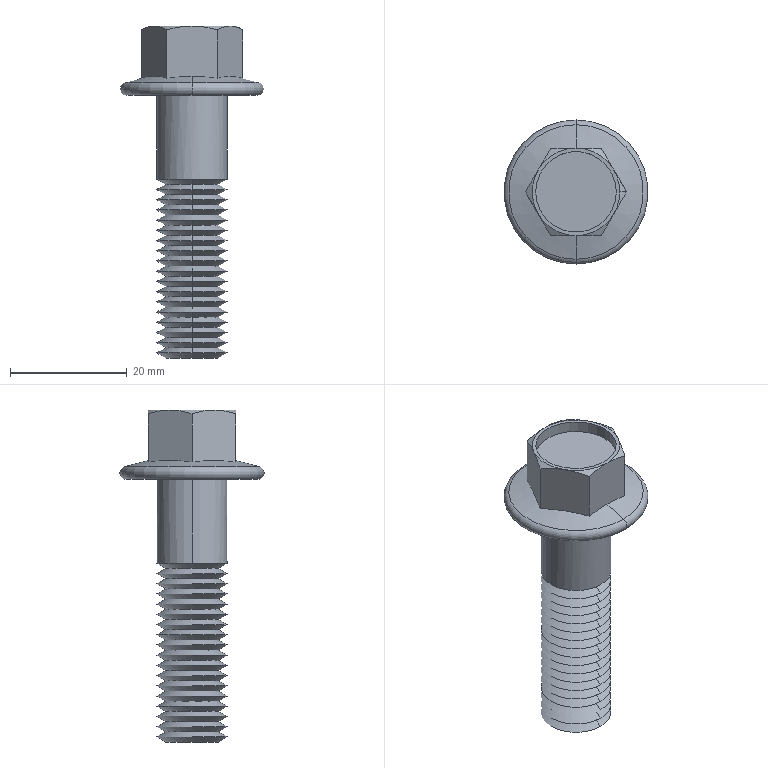Part | SolidWorks | features Cut 2, Boss 1, Extrusion 1, LPattern 1, RevCut 1, Revolution 1 | 1 solid | 129 faces | box 24.7 x 24.7 x 56.9 mm | volume 6988 mm3 | cone 79 | cylinder 38 | plane 10 | torus 2 | commonest cylinder face diameters 12 x36 13.8 x2